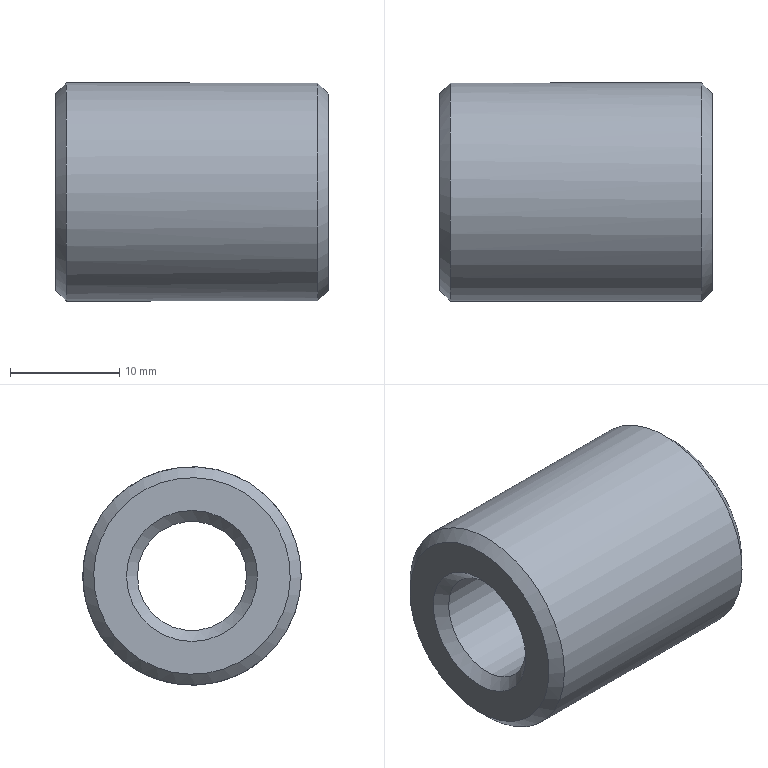Part | STEP file | SN10_015_004_BUCHA | 1 solid | 8 faces | box 25 x 20 x 20 mm | volume 5796 mm3 | cone 4 | plane 2 | cylinder 2 | commonest cylinder face diameters 10 x1 20 x1